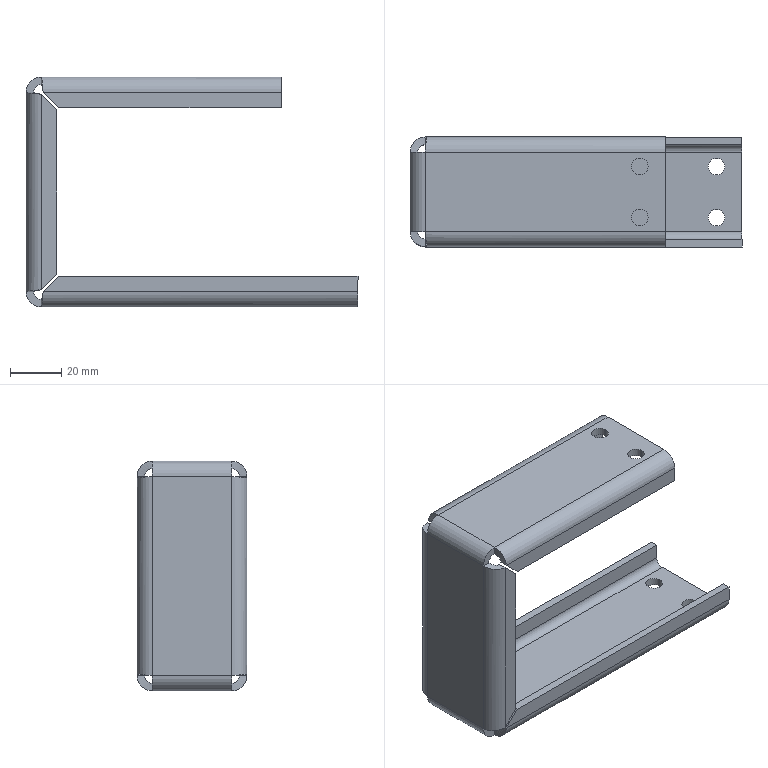Part | SolidWorks | features EdgeFlange 3, HoleWzd 2, MirrorPattern 2, FlatPattern 1, ICE 1, SMBaseFlange 1, SheetMetal 1 | 1 solid | 78 faces | box 130 x 43 x 90 mm | volume 51061 mm3 | plane 46 | cylinder 24 | spline 8 | commonest cylinder face diameters 6 x8 6.5 x8 12 x8